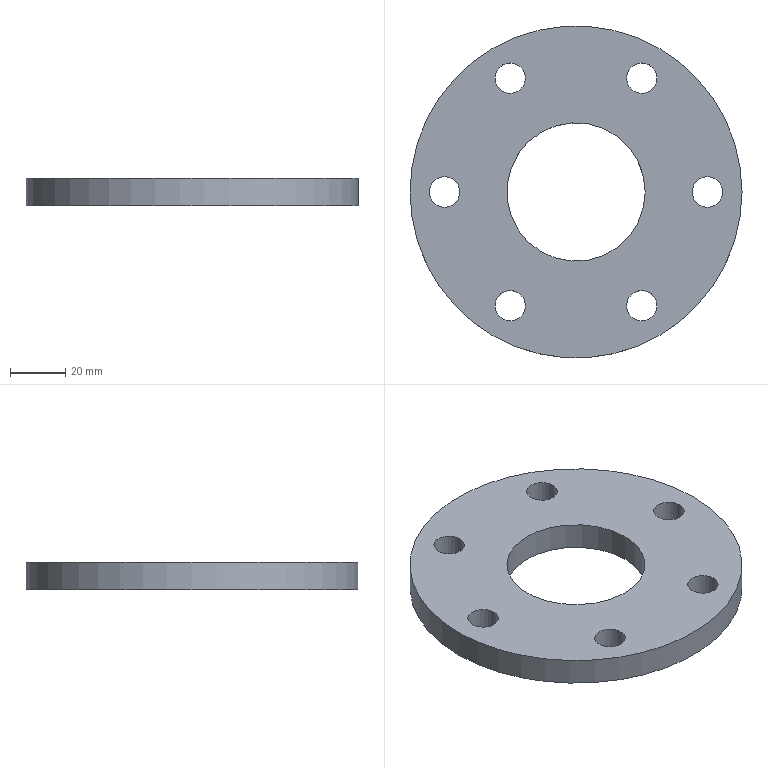Part | NX | 1 solid | 10 faces | box 120 x 120 x 10 mm | volume 87760 mm3 | cylinder 8 | plane 2 | commonest cylinder face diameters 11 x6 50 x1 120 x1
STEP:
#1=CARTESIAN_POINT('',(2953.931,208.53,-268.));
#2=VERTEX_POINT('',#1);
#3=CARTESIAN_POINT('',(2951.181,203.767,-268.));
#4=DIRECTION('',(0.,0.,1.));
#5=DIRECTION('',(0.5,0.866,0.));
#6=AXIS2_PLACEMENT_3D('',#3,#4,#5);
#7=CIRCLE('',#6,5.5);
#8=EDGE_CURVE('',#2,#2,#7,.T.);
#9=ORIENTED_EDGE('',*,*,#8,.T.);
#10=EDGE_LOOP('',(#9));
#11=FACE_BOUND('',#10,.T.);
#12=CARTESIAN_POINT('',(2953.931,208.53,-278.));
#13=VERTEX_POINT('',#12);
#14=CARTESIAN_POINT('',(2951.181,203.767,-278.));
#15=DIRECTION('',(0.,0.,1.));
#16=DIRECTION('',(0.5,0.866,0.));
#17=AXIS2_PLACEMENT_3D('',#14,#15,#16);
#18=CIRCLE('',#17,5.5);
#19=EDGE_CURVE('',#13,#13,#18,.T.);
#20=ORIENTED_EDGE('',*,*,#19,.F.);
#21=EDGE_LOOP('',(#20));
#22=FACE_BOUND('',#21,.T.);
#23=CARTESIAN_POINT('',(2951.181,203.767,-268.));
#24=DIRECTION('',(0.,0.,-1.));
#25=DIRECTION('',(1.,0.,0.));
#26=AXIS2_PLACEMENT_3D('',#23,#24,#25);
#27=CYLINDRICAL_SURFACE('',#26,5.5);
#28=ADVANCED_FACE('',(#11,#22),#27,.F.);
#29=CARTESIAN_POINT('',(2953.931,281.276,-268.));
#30=VERTEX_POINT('',#29);
#31=CARTESIAN_POINT('',(2951.181,286.04,-268.));
#32=DIRECTION('',(0.,0.,1.));
#33=DIRECTION('',(0.5,-0.866,0.));
#34=AXIS2_PLACEMENT_3D('',#31,#32,#33);
#35=CIRCLE('',#34,5.5);
#36=EDGE_CURVE('',#30,#30,#35,.T.);
#37=ORIENTED_EDGE('',*,*,#36,.T.);
#38=EDGE_LOOP('',(#37));
#39=FACE_BOUND('',#38,.T.);
#40=CARTESIAN_POINT('',(2953.931,281.276,-278.));
#41=VERTEX_POINT('',#40);
#42=CARTESIAN_POINT('',(2951.181,286.04,-278.));
#43=DIRECTION('',(0.,0.,1.));
#44=DIRECTION('',(0.5,-0.866,0.));
#45=AXIS2_PLACEMENT_3D('',#42,#43,#44);
#46=CIRCLE('',#45,5.5);
#47=EDGE_CURVE('',#41,#41,#46,.T.);
#48=ORIENTED_EDGE('',*,*,#47,.F.);
#49=EDGE_LOOP('',(#48));
#50=FACE_BOUND('',#49,.T.);
#51=CARTESIAN_POINT('',(2951.181,286.04,-268.));
#52=DIRECTION('',(0.,0.,-1.));
#53=DIRECTION('',(1.,0.,0.));
#54=AXIS2_PLACEMENT_3D('',#51,#52,#53);
#55=CYLINDRICAL_SURFACE('',#54,5.5);
#56=ADVANCED_FACE('',(#39,#50),#55,.F.);
#57=CARTESIAN_POINT('',(2999.931,244.903,-268.));
#58=VERTEX_POINT('',#57);
#59=CARTESIAN_POINT('',(2974.931,244.903,-268.));
#60=DIRECTION('',(0.,0.,1.));
#61=DIRECTION('',(1.,0.,0.));
#62=AXIS2_PLACEMENT_3D('',#59,#60,#61);
#63=CIRCLE('',#62,25.);
#64=EDGE_CURVE('',#58,#58,#63,.T.);
#65=ORIENTED_EDGE('',*,*,#64,.T.);
#66=EDGE_LOOP('',(#65));
#67=FACE_BOUND('',#66,.T.);
#68=CARTESIAN_POINT('',(2999.931,244.903,-278.));
#69=VERTEX_POINT('',#68);
#70=CARTESIAN_POINT('',(2974.931,244.903,-278.));
#71=DIRECTION('',(0.,0.,1.));
#72=DIRECTION('',(1.,0.,0.));
#73=AXIS2_PLACEMENT_3D('',#70,#71,#72);
#74=CIRCLE('',#73,25.);
#75=EDGE_CURVE('',#69,#69,#74,.T.);
#76=ORIENTED_EDGE('',*,*,#75,.F.);
#77=EDGE_LOOP('',(#76));
#78=FACE_BOUND('',#77,.T.);
#79=CARTESIAN_POINT('',(2974.931,244.903,-268.));
#80=DIRECTION('',(0.,0.,-1.));
#81=DIRECTION('',(1.,0.,0.));
#82=AXIS2_PLACEMENT_3D('',#79,#80,#81);
#83=CYLINDRICAL_SURFACE('',#82,25.);
#84=ADVANCED_FACE('',(#67,#78),#83,.F.);
#85=CARTESIAN_POINT('',(2995.931,208.53,-268.));
#86=VERTEX_POINT('',#85);
#87=CARTESIAN_POINT('',(2998.681,203.767,-268.));
#88=DIRECTION('',(0.,0.,1.));
#89=DIRECTION('',(-0.5,0.866,0.));
#90=AXIS2_PLACEMENT_3D('',#87,#88,#89);
#91=CIRCLE('',#90,5.5);
#92=EDGE_CURVE('',#86,#86,#91,.T.);
#93=ORIENTED_EDGE('',*,*,#92,.T.);
#94=EDGE_LOOP('',(#93));
#95=FACE_BOUND('',#94,.T.);
#96=CARTESIAN_POINT('',(2995.931,208.53,-278.));
#97=VERTEX_POINT('',#96);
#98=CARTESIAN_POINT('',(2998.681,203.767,-278.));
#99=DIRECTION('',(0.,0.,1.));
#100=DIRECTION('',(-0.5,0.866,0.));
#101=AXIS2_PLACEMENT_3D('',#98,#99,#100);
#102=CIRCLE('',#101,5.5);
#103=EDGE_CURVE('',#97,#97,#102,.T.);
#104=ORIENTED_EDGE('',*,*,#103,.F.);
#105=EDGE_LOOP('',(#104));
#106=FACE_BOUND('',#105,.T.);
#107=CARTESIAN_POINT('',(2998.681,203.767,-268.));
#108=DIRECTION('',(0.,0.,-1.));
#109=DIRECTION('',(1.,0.,0.));
#110=AXIS2_PLACEMENT_3D('',#107,#108,#109);
#111=CYLINDRICAL_SURFACE('',#110,5.5);
#112=ADVANCED_FACE('',(#95,#106),#111,.F.);
#113=CARTESIAN_POINT('',(2995.931,281.276,-268.));
#114=VERTEX_POINT('',#113);
#115=CARTESIAN_POINT('',(2998.681,286.04,-268.));
#116=DIRECTION('',(0.,0.,1.));
#117=DIRECTION('',(-0.5,-0.866,0.));
#118=AXIS2_PLACEMENT_3D('',#115,#116,#117);
#119=CIRCLE('',#118,5.5);
#120=EDGE_CURVE('',#114,#114,#119,.T.);
#121=ORIENTED_EDGE('',*,*,#120,.T.);
#122=EDGE_LOOP('',(#121));
#123=FACE_BOUND('',#122,.T.);
#124=CARTESIAN_POINT('',(2995.931,281.276,-278.));
#125=VERTEX_POINT('',#124);
#126=CARTESIAN_POINT('',(2998.681,286.04,-278.));
#127=DIRECTION('',(0.,0.,1.));
#128=DIRECTION('',(-0.5,-0.866,0.));
#129=AXIS2_PLACEMENT_3D('',#126,#127,#128);
#130=CIRCLE('',#129,5.5);
#131=EDGE_CURVE('',#125,#125,#130,.T.);
#132=ORIENTED_EDGE('',*,*,#131,.F.);
#133=EDGE_LOOP('',(#132));
#134=FACE_BOUND('',#133,.T.);
#135=CARTESIAN_POINT('',(2998.681,286.04,-268.));
#136=DIRECTION('',(0.,0.,-1.));
#137=DIRECTION('',(1.,0.,0.));
#138=AXIS2_PLACEMENT_3D('',#135,#136,#137);
#139=CYLINDRICAL_SURFACE('',#138,5.5);
#140=ADVANCED_FACE('',(#123,#134),#139,.F.);
#141=CARTESIAN_POINT('',(3016.931,244.903,-268.));
#142=VERTEX_POINT('',#141);
#143=CARTESIAN_POINT('',(3022.431,244.903,-268.));
#144=DIRECTION('',(0.,0.,1.));
#145=DIRECTION('',(-1.,0.,0.));
#146=AXIS2_PLACEMENT_3D('',#143,#144,#145);
#147=CIRCLE('',#146,5.5);
#148=EDGE_CURVE('',#142,#142,#147,.T.);
#149=ORIENTED_EDGE('',*,*,#148,.T.);
#150=EDGE_LOOP('',(#149));
#151=FACE_BOUND('',#150,.T.);
#152=CARTESIAN_POINT('',(3016.931,244.903,-278.));
#153=VERTEX_POINT('',#152);
#154=CARTESIAN_POINT('',(3022.431,244.903,-278.));
#155=DIRECTION('',(0.,0.,1.));
#156=DIRECTION('',(-1.,0.,0.));
#157=AXIS2_PLACEMENT_3D('',#154,#155,#156);
#158=CIRCLE('',#157,5.5);
#159=EDGE_CURVE('',#153,#153,#158,.T.);
#160=ORIENTED_EDGE('',*,*,#159,.F.);
#161=EDGE_LOOP('',(#160));
#162=FACE_BOUND('',#161,.T.);
#163=CARTESIAN_POINT('',(3022.431,244.903,-268.));
#164=DIRECTION('',(0.,0.,-1.));
#165=DIRECTION('',(1.,0.,0.));
#166=AXIS2_PLACEMENT_3D('',#163,#164,#165);
#167=CYLINDRICAL_SURFACE('',#166,5.5);
#168=ADVANCED_FACE('',(#151,#162),#167,.F.);
#169=CARTESIAN_POINT('',(3034.931,244.903,-268.));
#170=VERTEX_POINT('',#169);
#171=CARTESIAN_POINT('',(2974.931,244.903,-268.));
#172=DIRECTION('',(0.,0.,1.));
#173=DIRECTION('',(1.,0.,0.));
#174=AXIS2_PLACEMENT_3D('',#171,#172,#173);
#175=CIRCLE('',#174,60.);
#176=EDGE_CURVE('',#170,#170,#175,.T.);
#177=ORIENTED_EDGE('',*,*,#176,.F.);
#178=EDGE_LOOP('',(#177));
#179=FACE_BOUND('',#178,.T.);
#180=CARTESIAN_POINT('',(3034.931,244.903,-278.));
#181=VERTEX_POINT('',#180);
#182=CARTESIAN_POINT('',(2974.931,244.903,-278.));
#183=DIRECTION('',(0.,0.,1.));
#184=DIRECTION('',(1.,0.,0.));
#185=AXIS2_PLACEMENT_3D('',#182,#183,#184);
#186=CIRCLE('',#185,60.);
#187=EDGE_CURVE('',#181,#181,#186,.T.);
#188=ORIENTED_EDGE('',*,*,#187,.T.);
#189=EDGE_LOOP('',(#188));
#190=FACE_BOUND('',#189,.T.);
#191=CARTESIAN_POINT('',(2974.931,244.903,-268.));
#192=DIRECTION('',(0.,0.,-1.));
#193=DIRECTION('',(1.,0.,0.));
#194=AXIS2_PLACEMENT_3D('',#191,#192,#193);
#195=CYLINDRICAL_SURFACE('',#194,60.);
#196=ADVANCED_FACE('',(#179,#190),#195,.T.);
#197=CARTESIAN_POINT('',(2932.931,244.903,-268.));
#198=VERTEX_POINT('',#197);
#199=CARTESIAN_POINT('',(2927.431,244.903,-268.));
#200=DIRECTION('',(0.,0.,1.));
#201=DIRECTION('',(1.,0.,0.));
#202=AXIS2_PLACEMENT_3D('',#199,#200,#201);
#203=CIRCLE('',#202,5.5);
#204=EDGE_CURVE('',#198,#198,#203,.T.);
#205=ORIENTED_EDGE('',*,*,#204,.T.);
#206=EDGE_LOOP('',(#205));
#207=FACE_BOUND('',#206,.T.);
#208=CARTESIAN_POINT('',(2932.931,244.903,-278.));
#209=VERTEX_POINT('',#208);
#210=CARTESIAN_POINT('',(2927.431,244.903,-278.));
#211=DIRECTION('',(0.,0.,1.));
#212=DIRECTION('',(1.,0.,0.));
#213=AXIS2_PLACEMENT_3D('',#210,#211,#212);
#214=CIRCLE('',#213,5.5);
#215=EDGE_CURVE('',#209,#209,#214,.T.);
#216=ORIENTED_EDGE('',*,*,#215,.F.);
#217=EDGE_LOOP('',(#216));
#218=FACE_BOUND('',#217,.T.);
#219=CARTESIAN_POINT('',(2927.431,244.903,-268.));
#220=DIRECTION('',(0.,0.,-1.));
#221=DIRECTION('',(1.,0.,0.));
#222=AXIS2_PLACEMENT_3D('',#219,#220,#221);
#223=CYLINDRICAL_SURFACE('',#222,5.5);
#224=ADVANCED_FACE('',(#207,#218),#223,.F.);
#225=ORIENTED_EDGE('',*,*,#176,.T.);
#226=EDGE_LOOP('',(#225));
#227=FACE_BOUND('',#226,.T.);
#228=ORIENTED_EDGE('',*,*,#148,.F.);
#229=EDGE_LOOP('',(#228));
#230=FACE_BOUND('',#229,.T.);
#231=ORIENTED_EDGE('',*,*,#120,.F.);
#232=EDGE_LOOP('',(#231));
#233=FACE_BOUND('',#232,.T.);
#234=ORIENTED_EDGE('',*,*,#92,.F.);
#235=EDGE_LOOP('',(#234));
#236=FACE_BOUND('',#235,.T.);
#237=ORIENTED_EDGE('',*,*,#64,.F.);
#238=EDGE_LOOP('',(#237));
#239=FACE_BOUND('',#238,.T.);
#240=ORIENTED_EDGE('',*,*,#36,.F.);
#241=EDGE_LOOP('',(#240));
#242=FACE_BOUND('',#241,.T.);
#243=ORIENTED_EDGE('',*,*,#8,.F.);
#244=EDGE_LOOP('',(#243));
#245=FACE_BOUND('',#244,.T.);
#246=ORIENTED_EDGE('',*,*,#204,.F.);
#247=EDGE_LOOP('',(#246));
#248=FACE_BOUND('',#247,.T.);
#249=CARTESIAN_POINT('',(2998.681,244.903,-268.));
#250=DIRECTION('',(0.,0.,1.));
#251=DIRECTION('',(-1.,0.,0.));
#252=AXIS2_PLACEMENT_3D('',#249,#250,#251);
#253=PLANE('',#252);
#254=ADVANCED_FACE('',(#227,#230,#233,#236,#239,#242,#245,#248),#253,.T.);
#255=ORIENTED_EDGE('',*,*,#187,.F.);
#256=EDGE_LOOP('',(#255));
#257=FACE_BOUND('',#256,.T.);
#258=ORIENTED_EDGE('',*,*,#159,.T.);
#259=EDGE_LOOP('',(#258));
#260=FACE_BOUND('',#259,.T.);
#261=ORIENTED_EDGE('',*,*,#131,.T.);
#262=EDGE_LOOP('',(#261));
#263=FACE_BOUND('',#262,.T.);
#264=ORIENTED_EDGE('',*,*,#103,.T.);
#265=EDGE_LOOP('',(#264));
#266=FACE_BOUND('',#265,.T.);
#267=ORIENTED_EDGE('',*,*,#75,.T.);
#268=EDGE_LOOP('',(#267));
#269=FACE_BOUND('',#268,.T.);
#270=ORIENTED_EDGE('',*,*,#47,.T.);
#271=EDGE_LOOP('',(#270));
#272=FACE_BOUND('',#271,.T.);
#273=ORIENTED_EDGE('',*,*,#19,.T.);
#274=EDGE_LOOP('',(#273));
#275=FACE_BOUND('',#274,.T.);
#276=ORIENTED_EDGE('',*,*,#215,.T.);
#277=EDGE_LOOP('',(#276));
#278=FACE_BOUND('',#277,.T.);
#279=CARTESIAN_POINT('',(2998.681,244.903,-278.));
#280=DIRECTION('',(0.,0.,1.));
#281=DIRECTION('',(-1.,0.,0.));
#282=AXIS2_PLACEMENT_3D('',#279,#280,#281);
#283=PLANE('',#282);
#284=ADVANCED_FACE('',(#257,#260,#263,#266,#269,#272,#275,#278),#283,.F.);
#285=CLOSED_SHELL('',(#28,#56,#84,#112,#140,#168,#196,#224,#254,#284));
#286=MANIFOLD_SOLID_BREP('',#285);
#287=(LENGTH_UNIT()NAMED_UNIT(*)SI_UNIT(.MILLI.,.METRE.));
#288=UNCERTAINTY_MEASURE_WITH_UNIT(LENGTH_MEASURE(0.00002),#287,'','');
#289=(NAMED_UNIT(*)PLANE_ANGLE_UNIT()SI_UNIT($,.RADIAN.));
#290=PLANE_ANGLE_MEASURE_WITH_UNIT(PLANE_ANGLE_MEASURE(0.01745),#289);
#291=DIMENSIONAL_EXPONENTS(0.,0.,0.,0.,0.,0.,0.);
#292=(CONVERSION_BASED_UNIT('DEGREE',#290)NAMED_UNIT(#291)PLANE_ANGLE_UNIT());
#293=(NAMED_UNIT(*)SI_UNIT($,.STERADIAN.)SOLID_ANGLE_UNIT());
#294=(GEOMETRIC_REPRESENTATION_CONTEXT(3)GLOBAL_UNCERTAINTY_ASSIGNED_CONTEXT((#288))GLOBAL_UNIT_ASSIGNED_CONTEXT((#287,#292,#293))REPRESENTATION_CONTEXT('',''));
#295=ADVANCED_BREP_SHAPE_REPRESENTATION('',(#286),#294);